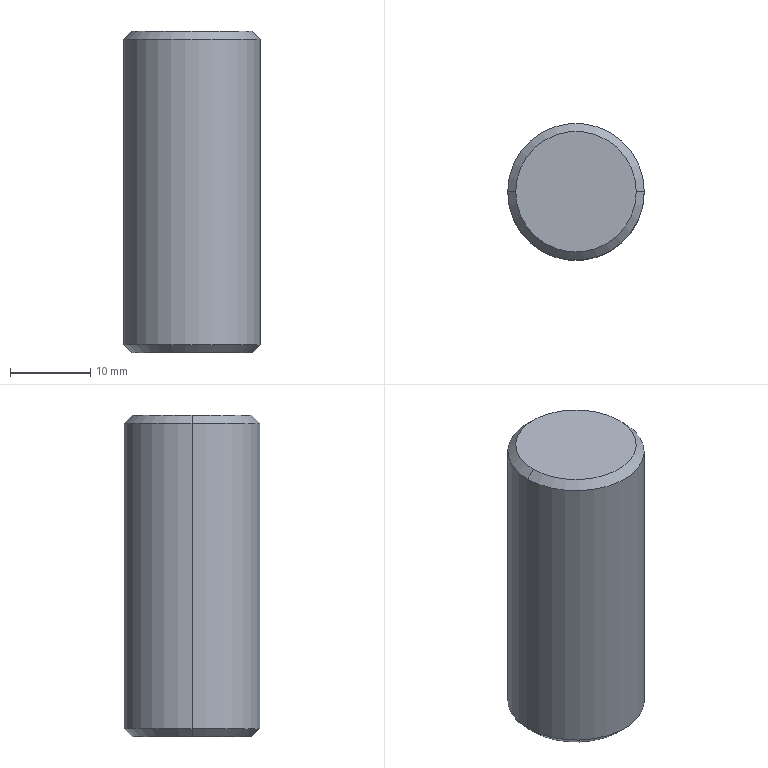Part | STEP file | ROLLER_DIA171V11 | 1 solid | 8 faces | box 17 x 17 x 40 mm | volume 9028 mm3 | cone 4 | cylinder 2 | plane 2 | commonest cylinder face diameters 17 x2
STEP:
#1=CARTESIAN_POINT('',(0.,0.,0.));
#2=DIRECTION('',(0.,0.,1.));
#3=DIRECTION('',(1.,0.,0.));
#4=AXIS2_PLACEMENT_3D('',#1,#2,#3);
#5=CARTESIAN_POINT('',(-7.5,0.,0.));
#6=VERTEX_POINT('',#5);
#7=CARTESIAN_POINT('',(7.5,0.,0.));
#8=VERTEX_POINT('',#7);
#9=CARTESIAN_POINT('',(0.,0.,0.));
#10=DIRECTION('',(0.,0.,-1.));
#11=DIRECTION('',(1.,0.,0.));
#12=AXIS2_PLACEMENT_3D('',#9,#10,#11);
#13=CIRCLE('',#12,7.5);
#14=CARTESIAN_POINT('',(0.,0.,1.));
#15=DIRECTION('',(0.,0.,1.));
#16=DIRECTION('',(1.,0.,0.));
#17=AXIS2_PLACEMENT_3D('',#14,#15,#16);
#18=CONICAL_SURFACE('',#17,8.5,0.7854);
#19=CARTESIAN_POINT('',(6.283,-1.));
#20=DIRECTION('',(-1.,0.));
#21=VECTOR('',#20,1.);
#22=LINE('',#19,#21);
#23=(GEOMETRIC_REPRESENTATION_CONTEXT(2)PARAMETRIC_REPRESENTATION_CONTEXT()REPRESENTATION_CONTEXT('',''));
#24=DEFINITIONAL_REPRESENTATION('',(#22),#23);
#25=PCURVE('',#18,#24);
#26=CARTESIAN_POINT('',(0.,0.,0.));
#27=DIRECTION('',(0.,0.,1.));
#28=DIRECTION('',(1.,0.,0.));
#29=AXIS2_PLACEMENT_3D('',#26,#27,#28);
#30=PLANE('',#29);
#31=CARTESIAN_POINT('',(7.5,0.));
#32=CARTESIAN_POINT('',(7.5,-12.99));
#33=CARTESIAN_POINT('',(-3.75,-6.495));
#34=CARTESIAN_POINT('',(-15.,0.));
#35=CARTESIAN_POINT('',(-3.75,6.495));
#36=CARTESIAN_POINT('',(7.5,12.99));
#37=CARTESIAN_POINT('',(7.5,0.));
#38=(BOUNDED_CURVE()B_SPLINE_CURVE(2,(#31,#32,#33,#34,#35,#36,#37),.UNSPECIFIED.,.T.,.F.)B_SPLINE_CURVE_WITH_KNOTS((1,2,2,2,2,1),(-2.094,0.,2.094,4.189,6.283,8.378),.UNSPECIFIED.)CURVE()GEOMETRIC_REPRESENTATION_ITEM()RATIONAL_B_SPLINE_CURVE((1.,0.5,1.,0.5,1.,0.5,1.))REPRESENTATION_ITEM(''));
#39=(GEOMETRIC_REPRESENTATION_CONTEXT(2)PARAMETRIC_REPRESENTATION_CONTEXT()REPRESENTATION_CONTEXT('',''));
#40=DEFINITIONAL_REPRESENTATION('',(#38),#39);
#41=PCURVE('',#30,#40);
#42=SURFACE_CURVE('',#13,(#25,#41),.PCURVE_S1.);
#43=EDGE_CURVE('',#6,#8,#42,.T.);
#44=ORIENTED_EDGE('',*,*,#43,.F.);
#45=CARTESIAN_POINT('',(-8.5,0.,1.));
#46=VERTEX_POINT('',#45);
#47=CARTESIAN_POINT('',(-8.5,0.,1.));
#48=DIRECTION('',(-0.7071,0.,0.7071));
#49=VECTOR('',#48,1.);
#50=LINE('',#47,#49);
#51=CARTESIAN_POINT('',(3.142,0.));
#52=DIRECTION('',(0.,1.));
#53=VECTOR('',#52,1.);
#54=LINE('',#51,#53);
#55=(GEOMETRIC_REPRESENTATION_CONTEXT(2)PARAMETRIC_REPRESENTATION_CONTEXT()REPRESENTATION_CONTEXT('',''));
#56=DEFINITIONAL_REPRESENTATION('',(#54),#55);
#57=PCURVE('',#18,#56);
#58=CARTESIAN_POINT('',(0.,0.,1.));
#59=DIRECTION('',(0.,0.,1.));
#60=DIRECTION('',(1.,0.,0.));
#61=AXIS2_PLACEMENT_3D('',#58,#59,#60);
#62=CONICAL_SURFACE('',#61,8.5,0.7854);
#63=CARTESIAN_POINT('',(3.142,0.));
#64=DIRECTION('',(0.,1.));
#65=VECTOR('',#64,1.);
#66=LINE('',#63,#65);
#67=(GEOMETRIC_REPRESENTATION_CONTEXT(2)PARAMETRIC_REPRESENTATION_CONTEXT()REPRESENTATION_CONTEXT('',''));
#68=DEFINITIONAL_REPRESENTATION('',(#66),#67);
#69=PCURVE('',#62,#68);
#70=SURFACE_CURVE('',#50,(#57,#69),.PCURVE_S1.);
#71=EDGE_CURVE('',#6,#46,#70,.T.);
#72=ORIENTED_EDGE('',*,*,#71,.T.);
#73=CARTESIAN_POINT('',(8.5,0.,1.));
#74=VERTEX_POINT('',#73);
#75=CARTESIAN_POINT('',(0.,0.,1.));
#76=DIRECTION('',(0.,0.,1.));
#77=DIRECTION('',(1.,0.,0.));
#78=AXIS2_PLACEMENT_3D('',#75,#76,#77);
#79=CIRCLE('',#78,8.5);
#80=CARTESIAN_POINT('',(0.,0.));
#81=DIRECTION('',(1.,0.));
#82=VECTOR('',#81,1.);
#83=LINE('',#80,#82);
#84=(GEOMETRIC_REPRESENTATION_CONTEXT(2)PARAMETRIC_REPRESENTATION_CONTEXT()REPRESENTATION_CONTEXT('',''));
#85=DEFINITIONAL_REPRESENTATION('',(#83),#84);
#86=PCURVE('',#18,#85);
#87=CARTESIAN_POINT('',(0.,0.,40.));
#88=DIRECTION('',(0.,0.,-1.));
#89=DIRECTION('',(-1.,0.,0.));
#90=AXIS2_PLACEMENT_3D('',#87,#88,#89);
#91=CYLINDRICAL_SURFACE('',#90,8.5);
#92=CARTESIAN_POINT('',(3.142,39.));
#93=DIRECTION('',(-1.,0.));
#94=VECTOR('',#93,1.);
#95=LINE('',#92,#94);
#96=(GEOMETRIC_REPRESENTATION_CONTEXT(2)PARAMETRIC_REPRESENTATION_CONTEXT()REPRESENTATION_CONTEXT('',''));
#97=DEFINITIONAL_REPRESENTATION('',(#95),#96);
#98=PCURVE('',#91,#97);
#99=SURFACE_CURVE('',#79,(#86,#98),.PCURVE_S1.);
#100=EDGE_CURVE('',#74,#46,#99,.T.);
#101=ORIENTED_EDGE('',*,*,#100,.F.);
#102=CARTESIAN_POINT('',(8.5,0.,1.));
#103=DIRECTION('',(0.7071,0.,0.7071));
#104=VECTOR('',#103,1.);
#105=LINE('',#102,#104);
#106=CARTESIAN_POINT('',(0.,0.));
#107=DIRECTION('',(0.,1.));
#108=VECTOR('',#107,1.);
#109=LINE('',#106,#108);
#110=(GEOMETRIC_REPRESENTATION_CONTEXT(2)PARAMETRIC_REPRESENTATION_CONTEXT()REPRESENTATION_CONTEXT('',''));
#111=DEFINITIONAL_REPRESENTATION('',(#109),#110);
#112=PCURVE('',#18,#111);
#113=CARTESIAN_POINT('',(6.283,0.));
#114=DIRECTION('',(0.,1.));
#115=VECTOR('',#114,1.);
#116=LINE('',#113,#115);
#117=(GEOMETRIC_REPRESENTATION_CONTEXT(2)PARAMETRIC_REPRESENTATION_CONTEXT()REPRESENTATION_CONTEXT('',''));
#118=DEFINITIONAL_REPRESENTATION('',(#116),#117);
#119=PCURVE('',#62,#118);
#120=SURFACE_CURVE('',#105,(#112,#119),.PCURVE_S1.);
#121=EDGE_CURVE('',#8,#74,#120,.T.);
#122=ORIENTED_EDGE('',*,*,#121,.F.);
#123=EDGE_LOOP('',(#44,#72,#101,#122));
#124=FACE_BOUND('',#123,.T.);
#125=ADVANCED_FACE('',(#124),#18,.T.);
#126=CARTESIAN_POINT('',(7.5,0.,40.));
#127=VERTEX_POINT('',#126);
#128=CARTESIAN_POINT('',(-7.5,0.,40.));
#129=VERTEX_POINT('',#128);
#130=CARTESIAN_POINT('',(0.,0.,40.));
#131=DIRECTION('',(0.,0.,1.));
#132=DIRECTION('',(1.,0.,0.));
#133=AXIS2_PLACEMENT_3D('',#130,#131,#132);
#134=CIRCLE('',#133,7.5);
#135=CARTESIAN_POINT('',(0.,0.,40.));
#136=DIRECTION('',(0.,0.,-1.));
#137=DIRECTION('',(-1.,0.,0.));
#138=AXIS2_PLACEMENT_3D('',#135,#136,#137);
#139=CONICAL_SURFACE('',#138,7.5,0.7854);
#140=CARTESIAN_POINT('',(3.142,0.));
#141=DIRECTION('',(-1.,0.));
#142=VECTOR('',#141,1.);
#143=LINE('',#140,#142);
#144=(GEOMETRIC_REPRESENTATION_CONTEXT(2)PARAMETRIC_REPRESENTATION_CONTEXT()REPRESENTATION_CONTEXT('',''));
#145=DEFINITIONAL_REPRESENTATION('',(#143),#144);
#146=PCURVE('',#139,#145);
#147=CARTESIAN_POINT('',(0.,0.,40.));
#148=DIRECTION('',(0.,0.,1.));
#149=DIRECTION('',(1.,0.,0.));
#150=AXIS2_PLACEMENT_3D('',#147,#148,#149);
#151=PLANE('',#150);
#152=CARTESIAN_POINT('',(0.,0.));
#153=DIRECTION('',(1.,0.));
#154=AXIS2_PLACEMENT_2D('',#152,#153);
#155=CIRCLE('',#154,7.5);
#156=(GEOMETRIC_REPRESENTATION_CONTEXT(2)PARAMETRIC_REPRESENTATION_CONTEXT()REPRESENTATION_CONTEXT('',''));
#157=DEFINITIONAL_REPRESENTATION('',(#155),#156);
#158=PCURVE('',#151,#157);
#159=SURFACE_CURVE('',#134,(#146,#158),.PCURVE_S1.);
#160=EDGE_CURVE('',#127,#129,#159,.T.);
#161=ORIENTED_EDGE('',*,*,#160,.F.);
#162=CARTESIAN_POINT('',(8.5,0.,39.));
#163=VERTEX_POINT('',#162);
#164=CARTESIAN_POINT('',(7.5,0.,40.));
#165=DIRECTION('',(0.7071,0.,-0.7071));
#166=VECTOR('',#165,1.);
#167=LINE('',#164,#166);
#168=CARTESIAN_POINT('',(3.142,0.));
#169=DIRECTION('',(0.,1.));
#170=VECTOR('',#169,1.);
#171=LINE('',#168,#170);
#172=(GEOMETRIC_REPRESENTATION_CONTEXT(2)PARAMETRIC_REPRESENTATION_CONTEXT()REPRESENTATION_CONTEXT('',''));
#173=DEFINITIONAL_REPRESENTATION('',(#171),#172);
#174=PCURVE('',#139,#173);
#175=CARTESIAN_POINT('',(0.,0.,40.));
#176=DIRECTION('',(0.,0.,-1.));
#177=DIRECTION('',(-1.,0.,0.));
#178=AXIS2_PLACEMENT_3D('',#175,#176,#177);
#179=CONICAL_SURFACE('',#178,7.5,0.7854);
#180=CARTESIAN_POINT('',(3.142,0.));
#181=DIRECTION('',(0.,1.));
#182=VECTOR('',#181,1.);
#183=LINE('',#180,#182);
#184=(GEOMETRIC_REPRESENTATION_CONTEXT(2)PARAMETRIC_REPRESENTATION_CONTEXT()REPRESENTATION_CONTEXT('',''));
#185=DEFINITIONAL_REPRESENTATION('',(#183),#184);
#186=PCURVE('',#179,#185);
#187=SURFACE_CURVE('',#167,(#174,#186),.PCURVE_S1.);
#188=EDGE_CURVE('',#127,#163,#187,.T.);
#189=ORIENTED_EDGE('',*,*,#188,.T.);
#190=CARTESIAN_POINT('',(-8.5,0.,39.));
#191=VERTEX_POINT('',#190);
#192=CARTESIAN_POINT('',(0.,0.,39.));
#193=DIRECTION('',(0.,0.,-1.));
#194=DIRECTION('',(1.,0.,0.));
#195=AXIS2_PLACEMENT_3D('',#192,#193,#194);
#196=CIRCLE('',#195,8.5);
#197=CARTESIAN_POINT('',(-3.142,1.));
#198=DIRECTION('',(1.,0.));
#199=VECTOR('',#198,1.);
#200=LINE('',#197,#199);
#201=(GEOMETRIC_REPRESENTATION_CONTEXT(2)PARAMETRIC_REPRESENTATION_CONTEXT()REPRESENTATION_CONTEXT('',''));
#202=DEFINITIONAL_REPRESENTATION('',(#200),#201);
#203=PCURVE('',#139,#202);
#204=CARTESIAN_POINT('',(-3.142,1.));
#205=DIRECTION('',(1.,0.));
#206=VECTOR('',#205,1.);
#207=LINE('',#204,#206);
#208=(GEOMETRIC_REPRESENTATION_CONTEXT(2)PARAMETRIC_REPRESENTATION_CONTEXT()REPRESENTATION_CONTEXT('',''));
#209=DEFINITIONAL_REPRESENTATION('',(#207),#208);
#210=PCURVE('',#91,#209);
#211=SURFACE_CURVE('',#196,(#203,#210),.PCURVE_S1.);
#212=EDGE_CURVE('',#191,#163,#211,.T.);
#213=ORIENTED_EDGE('',*,*,#212,.F.);
#214=CARTESIAN_POINT('',(-7.5,0.,40.));
#215=DIRECTION('',(-0.7071,0.,-0.7071));
#216=VECTOR('',#215,1.);
#217=LINE('',#214,#216);
#218=CARTESIAN_POINT('',(0.,0.));
#219=DIRECTION('',(0.,1.));
#220=VECTOR('',#219,1.);
#221=LINE('',#218,#220);
#222=(GEOMETRIC_REPRESENTATION_CONTEXT(2)PARAMETRIC_REPRESENTATION_CONTEXT()REPRESENTATION_CONTEXT('',''));
#223=DEFINITIONAL_REPRESENTATION('',(#221),#222);
#224=PCURVE('',#139,#223);
#225=CARTESIAN_POINT('',(6.283,0.));
#226=DIRECTION('',(0.,1.));
#227=VECTOR('',#226,1.);
#228=LINE('',#225,#227);
#229=(GEOMETRIC_REPRESENTATION_CONTEXT(2)PARAMETRIC_REPRESENTATION_CONTEXT()REPRESENTATION_CONTEXT('',''));
#230=DEFINITIONAL_REPRESENTATION('',(#228),#229);
#231=PCURVE('',#179,#230);
#232=SURFACE_CURVE('',#217,(#224,#231),.PCURVE_S1.);
#233=EDGE_CURVE('',#129,#191,#232,.T.);
#234=ORIENTED_EDGE('',*,*,#233,.F.);
#235=EDGE_LOOP('',(#161,#189,#213,#234));
#236=FACE_BOUND('',#235,.T.);
#237=ADVANCED_FACE('',(#236),#139,.T.);
#238=ORIENTED_EDGE('',*,*,#212,.T.);
#239=CARTESIAN_POINT('',(8.5,0.,40.));
#240=DIRECTION('',(0.,0.,-1.));
#241=VECTOR('',#240,1.);
#242=LINE('',#239,#241);
#243=CARTESIAN_POINT('',(3.142,0.));
#244=DIRECTION('',(0.,1.));
#245=VECTOR('',#244,1.);
#246=LINE('',#243,#245);
#247=(GEOMETRIC_REPRESENTATION_CONTEXT(2)PARAMETRIC_REPRESENTATION_CONTEXT()REPRESENTATION_CONTEXT('',''));
#248=DEFINITIONAL_REPRESENTATION('',(#246),#247);
#249=PCURVE('',#91,#248);
#250=CARTESIAN_POINT('',(0.,0.,40.));
#251=DIRECTION('',(0.,0.,-1.));
#252=DIRECTION('',(-1.,0.,0.));
#253=AXIS2_PLACEMENT_3D('',#250,#251,#252);
#254=CYLINDRICAL_SURFACE('',#253,8.5);
#255=CARTESIAN_POINT('',(3.142,0.));
#256=DIRECTION('',(0.,1.));
#257=VECTOR('',#256,1.);
#258=LINE('',#255,#257);
#259=(GEOMETRIC_REPRESENTATION_CONTEXT(2)PARAMETRIC_REPRESENTATION_CONTEXT()REPRESENTATION_CONTEXT('',''));
#260=DEFINITIONAL_REPRESENTATION('',(#258),#259);
#261=PCURVE('',#254,#260);
#262=SURFACE_CURVE('',#242,(#249,#261),.PCURVE_S1.);
#263=EDGE_CURVE('',#163,#74,#262,.T.);
#264=ORIENTED_EDGE('',*,*,#263,.T.);
#265=ORIENTED_EDGE('',*,*,#100,.T.);
#266=CARTESIAN_POINT('',(-8.5,0.,40.));
#267=DIRECTION('',(0.,0.,-1.));
#268=VECTOR('',#267,1.);
#269=LINE('',#266,#268);
#270=CARTESIAN_POINT('',(0.,0.));
#271=DIRECTION('',(0.,1.));
#272=VECTOR('',#271,1.);
#273=LINE('',#270,#272);
#274=(GEOMETRIC_REPRESENTATION_CONTEXT(2)PARAMETRIC_REPRESENTATION_CONTEXT()REPRESENTATION_CONTEXT('',''));
#275=DEFINITIONAL_REPRESENTATION('',(#273),#274);
#276=PCURVE('',#91,#275);
#277=CARTESIAN_POINT('',(6.283,0.));
#278=DIRECTION('',(0.,1.));
#279=VECTOR('',#278,1.);
#280=LINE('',#277,#279);
#281=(GEOMETRIC_REPRESENTATION_CONTEXT(2)PARAMETRIC_REPRESENTATION_CONTEXT()REPRESENTATION_CONTEXT('',''));
#282=DEFINITIONAL_REPRESENTATION('',(#280),#281);
#283=PCURVE('',#254,#282);
#284=SURFACE_CURVE('',#269,(#276,#283),.PCURVE_S1.);
#285=EDGE_CURVE('',#191,#46,#284,.T.);
#286=ORIENTED_EDGE('',*,*,#285,.F.);
#287=EDGE_LOOP('',(#238,#264,#265,#286));
#288=FACE_BOUND('',#287,.T.);
#289=ADVANCED_FACE('',(#288),#91,.T.);
#290=ORIENTED_EDGE('',*,*,#263,.F.);
#291=CARTESIAN_POINT('',(0.,0.,39.));
#292=DIRECTION('',(0.,0.,-1.));
#293=DIRECTION('',(1.,0.,0.));
#294=AXIS2_PLACEMENT_3D('',#291,#292,#293);
#295=CIRCLE('',#294,8.5);
#296=CARTESIAN_POINT('',(3.142,1.));
#297=DIRECTION('',(1.,0.));
#298=VECTOR('',#297,1.);
#299=LINE('',#296,#298);
#300=(GEOMETRIC_REPRESENTATION_CONTEXT(2)PARAMETRIC_REPRESENTATION_CONTEXT()REPRESENTATION_CONTEXT('',''));
#301=DEFINITIONAL_REPRESENTATION('',(#299),#300);
#302=PCURVE('',#254,#301);
#303=CARTESIAN_POINT('',(3.142,1.));
#304=DIRECTION('',(1.,0.));
#305=VECTOR('',#304,1.);
#306=LINE('',#303,#305);
#307=(GEOMETRIC_REPRESENTATION_CONTEXT(2)PARAMETRIC_REPRESENTATION_CONTEXT()REPRESENTATION_CONTEXT('',''));
#308=DEFINITIONAL_REPRESENTATION('',(#306),#307);
#309=PCURVE('',#179,#308);
#310=SURFACE_CURVE('',#295,(#302,#309),.PCURVE_S1.);
#311=EDGE_CURVE('',#163,#191,#310,.T.);
#312=ORIENTED_EDGE('',*,*,#311,.T.);
#313=ORIENTED_EDGE('',*,*,#285,.T.);
#314=CARTESIAN_POINT('',(0.,0.,1.));
#315=DIRECTION('',(0.,0.,1.));
#316=DIRECTION('',(1.,0.,0.));
#317=AXIS2_PLACEMENT_3D('',#314,#315,#316);
#318=CIRCLE('',#317,8.5);
#319=CARTESIAN_POINT('',(9.425,39.));
#320=DIRECTION('',(-1.,0.));
#321=VECTOR('',#320,1.);
#322=LINE('',#319,#321);
#323=(GEOMETRIC_REPRESENTATION_CONTEXT(2)PARAMETRIC_REPRESENTATION_CONTEXT()REPRESENTATION_CONTEXT('',''));
#324=DEFINITIONAL_REPRESENTATION('',(#322),#323);
#325=PCURVE('',#254,#324);
#326=CARTESIAN_POINT('',(0.,0.));
#327=DIRECTION('',(1.,0.));
#328=VECTOR('',#327,1.);
#329=LINE('',#326,#328);
#330=(GEOMETRIC_REPRESENTATION_CONTEXT(2)PARAMETRIC_REPRESENTATION_CONTEXT()REPRESENTATION_CONTEXT('',''));
#331=DEFINITIONAL_REPRESENTATION('',(#329),#330);
#332=PCURVE('',#62,#331);
#333=SURFACE_CURVE('',#318,(#325,#332),.PCURVE_S1.);
#334=EDGE_CURVE('',#46,#74,#333,.T.);
#335=ORIENTED_EDGE('',*,*,#334,.T.);
#336=EDGE_LOOP('',(#290,#312,#313,#335));
#337=FACE_BOUND('',#336,.T.);
#338=ADVANCED_FACE('',(#337),#254,.T.);
#339=CARTESIAN_POINT('',(0.,0.,40.));
#340=DIRECTION('',(0.,0.,1.));
#341=DIRECTION('',(1.,0.,0.));
#342=AXIS2_PLACEMENT_3D('',#339,#340,#341);
#343=CIRCLE('',#342,7.5);
#344=CARTESIAN_POINT('',(0.,0.));
#345=DIRECTION('',(1.,0.));
#346=AXIS2_PLACEMENT_2D('',#344,#345);
#347=CIRCLE('',#346,7.5);
#348=(GEOMETRIC_REPRESENTATION_CONTEXT(2)PARAMETRIC_REPRESENTATION_CONTEXT()REPRESENTATION_CONTEXT('',''));
#349=DEFINITIONAL_REPRESENTATION('',(#347),#348);
#350=PCURVE('',#151,#349);
#351=CARTESIAN_POINT('',(9.425,0.));
#352=DIRECTION('',(-1.,0.));
#353=VECTOR('',#352,1.);
#354=LINE('',#351,#353);
#355=(GEOMETRIC_REPRESENTATION_CONTEXT(2)PARAMETRIC_REPRESENTATION_CONTEXT()REPRESENTATION_CONTEXT('',''));
#356=DEFINITIONAL_REPRESENTATION('',(#354),#355);
#357=PCURVE('',#179,#356);
#358=SURFACE_CURVE('',#343,(#350,#357),.PCURVE_S1.);
#359=EDGE_CURVE('',#129,#127,#358,.T.);
#360=ORIENTED_EDGE('',*,*,#359,.T.);
#361=ORIENTED_EDGE('',*,*,#160,.T.);
#362=EDGE_LOOP('',(#360,#361));
#363=FACE_BOUND('',#362,.T.);
#364=ADVANCED_FACE('',(#363),#151,.T.);
#365=CARTESIAN_POINT('',(0.,0.,0.));
#366=DIRECTION('',(0.,0.,-1.));
#367=DIRECTION('',(1.,0.,0.));
#368=AXIS2_PLACEMENT_3D('',#365,#366,#367);
#369=CIRCLE('',#368,7.5);
#370=CARTESIAN_POINT('',(7.5,0.));
#371=CARTESIAN_POINT('',(7.5,-12.99));
#372=CARTESIAN_POINT('',(-3.75,-6.495));
#373=CARTESIAN_POINT('',(-15.,0.));
#374=CARTESIAN_POINT('',(-3.75,6.495));
#375=CARTESIAN_POINT('',(7.5,12.99));
#376=CARTESIAN_POINT('',(7.5,0.));
#377=(BOUNDED_CURVE()B_SPLINE_CURVE(2,(#370,#371,#372,#373,#374,#375,#376),.UNSPECIFIED.,.T.,.F.)B_SPLINE_CURVE_WITH_KNOTS((1,2,2,2,2,1),(-2.094,0.,2.094,4.189,6.283,8.378),.UNSPECIFIED.)CURVE()GEOMETRIC_REPRESENTATION_ITEM()RATIONAL_B_SPLINE_CURVE((1.,0.5,1.,0.5,1.,0.5,1.))REPRESENTATION_ITEM(''));
#378=(GEOMETRIC_REPRESENTATION_CONTEXT(2)PARAMETRIC_REPRESENTATION_CONTEXT()REPRESENTATION_CONTEXT('',''));
#379=DEFINITIONAL_REPRESENTATION('',(#377),#378);
#380=PCURVE('',#30,#379);
#381=CARTESIAN_POINT('',(6.283,-1.));
#382=DIRECTION('',(-1.,0.));
#383=VECTOR('',#382,1.);
#384=LINE('',#381,#383);
#385=(GEOMETRIC_REPRESENTATION_CONTEXT(2)PARAMETRIC_REPRESENTATION_CONTEXT()REPRESENTATION_CONTEXT('',''));
#386=DEFINITIONAL_REPRESENTATION('',(#384),#385);
#387=PCURVE('',#62,#386);
#388=SURFACE_CURVE('',#369,(#380,#387),.PCURVE_S1.);
#389=EDGE_CURVE('',#8,#6,#388,.T.);
#390=ORIENTED_EDGE('',*,*,#389,.T.);
#391=ORIENTED_EDGE('',*,*,#43,.T.);
#392=EDGE_LOOP('',(#390,#391));
#393=FACE_BOUND('',#392,.T.);
#394=ADVANCED_FACE('',(#393),#30,.F.);
#395=ORIENTED_EDGE('',*,*,#188,.F.);
#396=ORIENTED_EDGE('',*,*,#359,.F.);
#397=ORIENTED_EDGE('',*,*,#233,.T.);
#398=ORIENTED_EDGE('',*,*,#311,.F.);
#399=EDGE_LOOP('',(#395,#396,#397,#398));
#400=FACE_BOUND('',#399,.T.);
#401=ADVANCED_FACE('',(#400),#179,.T.);
#402=ORIENTED_EDGE('',*,*,#71,.F.);
#403=ORIENTED_EDGE('',*,*,#389,.F.);
#404=ORIENTED_EDGE('',*,*,#121,.T.);
#405=ORIENTED_EDGE('',*,*,#334,.F.);
#406=EDGE_LOOP('',(#402,#403,#404,#405));
#407=FACE_BOUND('',#406,.T.);
#408=ADVANCED_FACE('',(#407),#62,.T.);
#409=CLOSED_SHELL('',(#125,#237,#289,#338,#364,#394,#401,#408));
#410=MANIFOLD_SOLID_BREP('',#409);
#411=(LENGTH_UNIT()NAMED_UNIT(*)SI_UNIT(.MILLI.,.METRE.));
#412=UNCERTAINTY_MEASURE_WITH_UNIT(LENGTH_MEASURE(0.0000001),#411,'','');
#413=(NAMED_UNIT(*)PLANE_ANGLE_UNIT()SI_UNIT($,.RADIAN.));
#414=(NAMED_UNIT(*)SI_UNIT($,.STERADIAN.)SOLID_ANGLE_UNIT());
#415=(GEOMETRIC_REPRESENTATION_CONTEXT(3)GLOBAL_UNCERTAINTY_ASSIGNED_CONTEXT((#412))GLOBAL_UNIT_ASSIGNED_CONTEXT((#411,#413,#414))REPRESENTATION_CONTEXT('',''));
#416=ADVANCED_BREP_SHAPE_REPRESENTATION('',(#4,#410),#415);